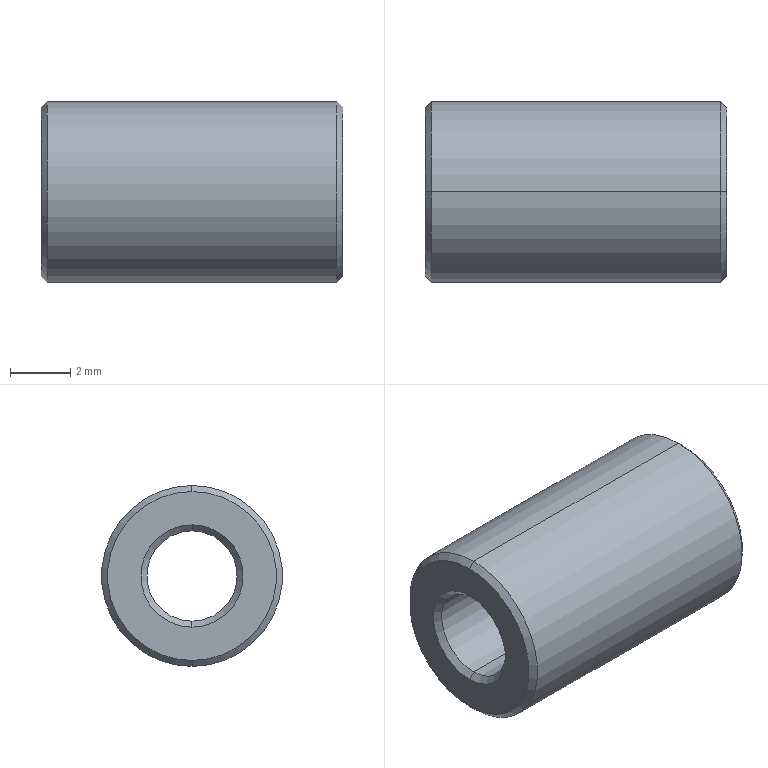Part | STEP file | KNCLSS3-8-10 | 1 solid | 14 faces | box 10 x 6 x 6 mm | volume 210.927 mm3 | cone 8 | cylinder 4 | plane 2 | commonest cylinder face diameters 3 x2 6 x2
STEP:
#1=CARTESIAN_POINT('',(0.,0.,0.));
#2=DIRECTION('',(0.,0.,1.));
#3=DIRECTION('',(1.,0.,0.));
#4=AXIS2_PLACEMENT_3D('',#1,#2,#3);
#5=CARTESIAN_POINT('',(9.8,0.,-1.5));
#6=VERTEX_POINT('',#5);
#7=CARTESIAN_POINT('',(10.,0.,-1.7));
#8=VERTEX_POINT('',#7);
#9=CARTESIAN_POINT('',(9.8,0.,-1.5));
#10=DIRECTION('',(0.7071,0.,-0.7071));
#11=VECTOR('',#10,1.);
#12=LINE('',#9,#11);
#13=CARTESIAN_POINT('',(9.8,0.,0.));
#14=DIRECTION('',(1.,0.,0.));
#15=DIRECTION('',(0.,0.,-1.));
#16=AXIS2_PLACEMENT_3D('',#13,#14,#15);
#17=CONICAL_SURFACE('',#16,1.5,0.7854);
#18=CARTESIAN_POINT('',(6.283,0.));
#19=DIRECTION('',(0.,1.));
#20=VECTOR('',#19,1.);
#21=LINE('',#18,#20);
#22=(GEOMETRIC_REPRESENTATION_CONTEXT(2)PARAMETRIC_REPRESENTATION_CONTEXT()REPRESENTATION_CONTEXT('',''));
#23=DEFINITIONAL_REPRESENTATION('',(#21),#22);
#24=PCURVE('',#17,#23);
#25=CARTESIAN_POINT('',(9.8,0.,0.));
#26=DIRECTION('',(1.,0.,0.));
#27=DIRECTION('',(0.,0.,-1.));
#28=AXIS2_PLACEMENT_3D('',#25,#26,#27);
#29=CONICAL_SURFACE('',#28,1.5,0.7854);
#30=CARTESIAN_POINT('',(0.,0.));
#31=DIRECTION('',(0.,1.));
#32=VECTOR('',#31,1.);
#33=LINE('',#30,#32);
#34=(GEOMETRIC_REPRESENTATION_CONTEXT(2)PARAMETRIC_REPRESENTATION_CONTEXT()REPRESENTATION_CONTEXT('',''));
#35=DEFINITIONAL_REPRESENTATION('',(#33),#34);
#36=PCURVE('',#29,#35);
#37=SURFACE_CURVE('',#12,(#24,#36),.PCURVE_S1.);
#38=EDGE_CURVE('',#6,#8,#37,.T.);
#39=ORIENTED_EDGE('',*,*,#38,.T.);
#40=CARTESIAN_POINT('',(10.,0.,1.7));
#41=VERTEX_POINT('',#40);
#42=CARTESIAN_POINT('',(10.,0.,0.));
#43=DIRECTION('',(1.,0.,0.));
#44=DIRECTION('',(0.,0.,-1.));
#45=AXIS2_PLACEMENT_3D('',#42,#43,#44);
#46=CIRCLE('',#45,1.7);
#47=CARTESIAN_POINT('',(0.,0.2));
#48=DIRECTION('',(1.,0.));
#49=VECTOR('',#48,1.);
#50=LINE('',#47,#49);
#51=(GEOMETRIC_REPRESENTATION_CONTEXT(2)PARAMETRIC_REPRESENTATION_CONTEXT()REPRESENTATION_CONTEXT('',''));
#52=DEFINITIONAL_REPRESENTATION('',(#50),#51);
#53=PCURVE('',#17,#52);
#54=CARTESIAN_POINT('',(10.,3.8,0.));
#55=DIRECTION('',(-1.,0.,0.));
#56=DIRECTION('',(0.,0.,1.));
#57=AXIS2_PLACEMENT_3D('',#54,#55,#56);
#58=PLANE('',#57);
#59=CARTESIAN_POINT('',(-1.7,-3.8));
#60=CARTESIAN_POINT('',(-1.7,-0.8555));
#61=CARTESIAN_POINT('',(0.85,-2.328));
#62=CARTESIAN_POINT('',(3.4,-3.8));
#63=CARTESIAN_POINT('',(0.85,-5.272));
#64=CARTESIAN_POINT('',(-1.7,-6.744));
#65=CARTESIAN_POINT('',(-1.7,-3.8));
#66=(BOUNDED_CURVE()B_SPLINE_CURVE(2,(#59,#60,#61,#62,#63,#64,#65),.UNSPECIFIED.,.T.,.F.)B_SPLINE_CURVE_WITH_KNOTS((1,2,2,2,2,1),(-2.094,0.,2.094,4.189,6.283,8.378),.UNSPECIFIED.)CURVE()GEOMETRIC_REPRESENTATION_ITEM()RATIONAL_B_SPLINE_CURVE((1.,0.5,1.,0.5,1.,0.5,1.))REPRESENTATION_ITEM(''));
#67=(GEOMETRIC_REPRESENTATION_CONTEXT(2)PARAMETRIC_REPRESENTATION_CONTEXT()REPRESENTATION_CONTEXT('',''));
#68=DEFINITIONAL_REPRESENTATION('',(#66),#67);
#69=PCURVE('',#58,#68);
#70=SURFACE_CURVE('',#46,(#53,#69),.PCURVE_S1.);
#71=EDGE_CURVE('',#41,#8,#70,.T.);
#72=ORIENTED_EDGE('',*,*,#71,.F.);
#73=CARTESIAN_POINT('',(9.8,0.,1.5));
#74=VERTEX_POINT('',#73);
#75=CARTESIAN_POINT('',(9.8,0.,1.5));
#76=DIRECTION('',(0.7071,0.,0.7071));
#77=VECTOR('',#76,1.);
#78=LINE('',#75,#77);
#79=CARTESIAN_POINT('',(3.142,0.));
#80=DIRECTION('',(0.,1.));
#81=VECTOR('',#80,1.);
#82=LINE('',#79,#81);
#83=(GEOMETRIC_REPRESENTATION_CONTEXT(2)PARAMETRIC_REPRESENTATION_CONTEXT()REPRESENTATION_CONTEXT('',''));
#84=DEFINITIONAL_REPRESENTATION('',(#82),#83);
#85=PCURVE('',#17,#84);
#86=CARTESIAN_POINT('',(3.142,0.));
#87=DIRECTION('',(0.,1.));
#88=VECTOR('',#87,1.);
#89=LINE('',#86,#88);
#90=(GEOMETRIC_REPRESENTATION_CONTEXT(2)PARAMETRIC_REPRESENTATION_CONTEXT()REPRESENTATION_CONTEXT('',''));
#91=DEFINITIONAL_REPRESENTATION('',(#89),#90);
#92=PCURVE('',#29,#91);
#93=SURFACE_CURVE('',#78,(#85,#92),.PCURVE_S1.);
#94=EDGE_CURVE('',#74,#41,#93,.T.);
#95=ORIENTED_EDGE('',*,*,#94,.F.);
#96=CARTESIAN_POINT('',(9.8,0.,0.));
#97=DIRECTION('',(1.,0.,0.));
#98=DIRECTION('',(0.,0.,-1.));
#99=AXIS2_PLACEMENT_3D('',#96,#97,#98);
#100=CIRCLE('',#99,1.5);
#101=CARTESIAN_POINT('',(0.,0.));
#102=DIRECTION('',(1.,0.));
#103=VECTOR('',#102,1.);
#104=LINE('',#101,#103);
#105=(GEOMETRIC_REPRESENTATION_CONTEXT(2)PARAMETRIC_REPRESENTATION_CONTEXT()REPRESENTATION_CONTEXT('',''));
#106=DEFINITIONAL_REPRESENTATION('',(#104),#105);
#107=PCURVE('',#17,#106);
#108=CARTESIAN_POINT('',(10.,0.,0.));
#109=DIRECTION('',(1.,0.,0.));
#110=DIRECTION('',(0.,0.,-1.));
#111=AXIS2_PLACEMENT_3D('',#108,#109,#110);
#112=CYLINDRICAL_SURFACE('',#111,1.5);
#113=CARTESIAN_POINT('',(0.,-0.2));
#114=DIRECTION('',(1.,0.));
#115=VECTOR('',#114,1.);
#116=LINE('',#113,#115);
#117=(GEOMETRIC_REPRESENTATION_CONTEXT(2)PARAMETRIC_REPRESENTATION_CONTEXT()REPRESENTATION_CONTEXT('',''));
#118=DEFINITIONAL_REPRESENTATION('',(#116),#117);
#119=PCURVE('',#112,#118);
#120=SURFACE_CURVE('',#100,(#107,#119),.PCURVE_S1.);
#121=EDGE_CURVE('',#74,#6,#120,.T.);
#122=ORIENTED_EDGE('',*,*,#121,.T.);
#123=EDGE_LOOP('',(#39,#72,#95,#122));
#124=FACE_BOUND('',#123,.F.);
#125=ADVANCED_FACE('',(#124),#17,.F.);
#126=CARTESIAN_POINT('',(0.2,0.,-1.5));
#127=VERTEX_POINT('',#126);
#128=CARTESIAN_POINT('',(10.,0.,-1.5));
#129=DIRECTION('',(1.,0.,0.));
#130=VECTOR('',#129,1.);
#131=LINE('',#128,#130);
#132=CARTESIAN_POINT('',(6.283,0.));
#133=DIRECTION('',(0.,1.));
#134=VECTOR('',#133,1.);
#135=LINE('',#132,#134);
#136=(GEOMETRIC_REPRESENTATION_CONTEXT(2)PARAMETRIC_REPRESENTATION_CONTEXT()REPRESENTATION_CONTEXT('',''));
#137=DEFINITIONAL_REPRESENTATION('',(#135),#136);
#138=PCURVE('',#112,#137);
#139=CARTESIAN_POINT('',(10.,0.,0.));
#140=DIRECTION('',(1.,0.,0.));
#141=DIRECTION('',(0.,0.,-1.));
#142=AXIS2_PLACEMENT_3D('',#139,#140,#141);
#143=CYLINDRICAL_SURFACE('',#142,1.5);
#144=CARTESIAN_POINT('',(0.,0.));
#145=DIRECTION('',(0.,1.));
#146=VECTOR('',#145,1.);
#147=LINE('',#144,#146);
#148=(GEOMETRIC_REPRESENTATION_CONTEXT(2)PARAMETRIC_REPRESENTATION_CONTEXT()REPRESENTATION_CONTEXT('',''));
#149=DEFINITIONAL_REPRESENTATION('',(#147),#148);
#150=PCURVE('',#143,#149);
#151=SURFACE_CURVE('',#131,(#138,#150),.PCURVE_S1.);
#152=EDGE_CURVE('',#127,#6,#151,.T.);
#153=ORIENTED_EDGE('',*,*,#152,.T.);
#154=ORIENTED_EDGE('',*,*,#121,.F.);
#155=CARTESIAN_POINT('',(0.2,0.,1.5));
#156=VERTEX_POINT('',#155);
#157=CARTESIAN_POINT('',(10.,0.,1.5));
#158=DIRECTION('',(1.,0.,0.));
#159=VECTOR('',#158,1.);
#160=LINE('',#157,#159);
#161=CARTESIAN_POINT('',(3.142,0.));
#162=DIRECTION('',(0.,1.));
#163=VECTOR('',#162,1.);
#164=LINE('',#161,#163);
#165=(GEOMETRIC_REPRESENTATION_CONTEXT(2)PARAMETRIC_REPRESENTATION_CONTEXT()REPRESENTATION_CONTEXT('',''));
#166=DEFINITIONAL_REPRESENTATION('',(#164),#165);
#167=PCURVE('',#112,#166);
#168=CARTESIAN_POINT('',(3.142,0.));
#169=DIRECTION('',(0.,1.));
#170=VECTOR('',#169,1.);
#171=LINE('',#168,#170);
#172=(GEOMETRIC_REPRESENTATION_CONTEXT(2)PARAMETRIC_REPRESENTATION_CONTEXT()REPRESENTATION_CONTEXT('',''));
#173=DEFINITIONAL_REPRESENTATION('',(#171),#172);
#174=PCURVE('',#143,#173);
#175=SURFACE_CURVE('',#160,(#167,#174),.PCURVE_S1.);
#176=EDGE_CURVE('',#156,#74,#175,.T.);
#177=ORIENTED_EDGE('',*,*,#176,.F.);
#178=CARTESIAN_POINT('',(0.2,0.,0.));
#179=DIRECTION('',(1.,0.,0.));
#180=DIRECTION('',(0.,0.,-1.));
#181=AXIS2_PLACEMENT_3D('',#178,#179,#180);
#182=CIRCLE('',#181,1.5);
#183=CARTESIAN_POINT('',(0.,-9.8));
#184=DIRECTION('',(1.,0.));
#185=VECTOR('',#184,1.);
#186=LINE('',#183,#185);
#187=(GEOMETRIC_REPRESENTATION_CONTEXT(2)PARAMETRIC_REPRESENTATION_CONTEXT()REPRESENTATION_CONTEXT('',''));
#188=DEFINITIONAL_REPRESENTATION('',(#186),#187);
#189=PCURVE('',#112,#188);
#190=CARTESIAN_POINT('',(0.,0.,0.));
#191=DIRECTION('',(-1.,0.,0.));
#192=DIRECTION('',(0.,0.,1.));
#193=AXIS2_PLACEMENT_3D('',#190,#191,#192);
#194=CONICAL_SURFACE('',#193,1.7,0.7854);
#195=CARTESIAN_POINT('',(9.425,-0.2));
#196=DIRECTION('',(-1.,0.));
#197=VECTOR('',#196,1.);
#198=LINE('',#195,#197);
#199=(GEOMETRIC_REPRESENTATION_CONTEXT(2)PARAMETRIC_REPRESENTATION_CONTEXT()REPRESENTATION_CONTEXT('',''));
#200=DEFINITIONAL_REPRESENTATION('',(#198),#199);
#201=PCURVE('',#194,#200);
#202=SURFACE_CURVE('',#182,(#189,#201),.PCURVE_S1.);
#203=EDGE_CURVE('',#156,#127,#202,.T.);
#204=ORIENTED_EDGE('',*,*,#203,.T.);
#205=EDGE_LOOP('',(#153,#154,#177,#204));
#206=FACE_BOUND('',#205,.F.);
#207=ADVANCED_FACE('',(#206),#112,.F.);
#208=CARTESIAN_POINT('',(0.,0.,1.7));
#209=VERTEX_POINT('',#208);
#210=CARTESIAN_POINT('',(0.,0.,1.7));
#211=DIRECTION('',(-0.7071,0.,0.7071));
#212=VECTOR('',#211,1.);
#213=LINE('',#210,#212);
#214=CARTESIAN_POINT('',(6.283,0.));
#215=DIRECTION('',(0.,1.));
#216=VECTOR('',#215,1.);
#217=LINE('',#214,#216);
#218=(GEOMETRIC_REPRESENTATION_CONTEXT(2)PARAMETRIC_REPRESENTATION_CONTEXT()REPRESENTATION_CONTEXT('',''));
#219=DEFINITIONAL_REPRESENTATION('',(#217),#218);
#220=PCURVE('',#194,#219);
#221=CARTESIAN_POINT('',(0.,0.,0.));
#222=DIRECTION('',(-1.,0.,0.));
#223=DIRECTION('',(0.,0.,1.));
#224=AXIS2_PLACEMENT_3D('',#221,#222,#223);
#225=CONICAL_SURFACE('',#224,1.7,0.7854);
#226=CARTESIAN_POINT('',(0.,0.));
#227=DIRECTION('',(0.,1.));
#228=VECTOR('',#227,1.);
#229=LINE('',#226,#228);
#230=(GEOMETRIC_REPRESENTATION_CONTEXT(2)PARAMETRIC_REPRESENTATION_CONTEXT()REPRESENTATION_CONTEXT('',''));
#231=DEFINITIONAL_REPRESENTATION('',(#229),#230);
#232=PCURVE('',#225,#231);
#233=SURFACE_CURVE('',#213,(#220,#232),.PCURVE_S1.);
#234=EDGE_CURVE('',#156,#209,#233,.T.);
#235=ORIENTED_EDGE('',*,*,#234,.T.);
#236=CARTESIAN_POINT('',(0.,0.,-1.7));
#237=VERTEX_POINT('',#236);
#238=CARTESIAN_POINT('',(0.,0.,0.));
#239=DIRECTION('',(1.,0.,0.));
#240=DIRECTION('',(0.,0.,-1.));
#241=AXIS2_PLACEMENT_3D('',#238,#239,#240);
#242=CIRCLE('',#241,1.7);
#243=CARTESIAN_POINT('',(9.425,0.));
#244=DIRECTION('',(-1.,0.));
#245=VECTOR('',#244,1.);
#246=LINE('',#243,#245);
#247=(GEOMETRIC_REPRESENTATION_CONTEXT(2)PARAMETRIC_REPRESENTATION_CONTEXT()REPRESENTATION_CONTEXT('',''));
#248=DEFINITIONAL_REPRESENTATION('',(#246),#247);
#249=PCURVE('',#194,#248);
#250=CARTESIAN_POINT('',(0.,0.,0.));
#251=DIRECTION('',(1.,0.,0.));
#252=DIRECTION('',(0.,0.,-1.));
#253=AXIS2_PLACEMENT_3D('',#250,#251,#252);
#254=PLANE('',#253);
#255=CARTESIAN_POINT('',(0.,0.));
#256=DIRECTION('',(1.,0.));
#257=AXIS2_PLACEMENT_2D('',#255,#256);
#258=CIRCLE('',#257,1.7);
#259=(GEOMETRIC_REPRESENTATION_CONTEXT(2)PARAMETRIC_REPRESENTATION_CONTEXT()REPRESENTATION_CONTEXT('',''));
#260=DEFINITIONAL_REPRESENTATION('',(#258),#259);
#261=PCURVE('',#254,#260);
#262=SURFACE_CURVE('',#242,(#249,#261),.PCURVE_S1.);
#263=EDGE_CURVE('',#209,#237,#262,.T.);
#264=ORIENTED_EDGE('',*,*,#263,.T.);
#265=CARTESIAN_POINT('',(0.,0.,-1.7));
#266=DIRECTION('',(-0.7071,0.,-0.7071));
#267=VECTOR('',#266,1.);
#268=LINE('',#265,#267);
#269=CARTESIAN_POINT('',(3.142,0.));
#270=DIRECTION('',(0.,1.));
#271=VECTOR('',#270,1.);
#272=LINE('',#269,#271);
#273=(GEOMETRIC_REPRESENTATION_CONTEXT(2)PARAMETRIC_REPRESENTATION_CONTEXT()REPRESENTATION_CONTEXT('',''));
#274=DEFINITIONAL_REPRESENTATION('',(#272),#273);
#275=PCURVE('',#194,#274);
#276=CARTESIAN_POINT('',(3.142,0.));
#277=DIRECTION('',(0.,1.));
#278=VECTOR('',#277,1.);
#279=LINE('',#276,#278);
#280=(GEOMETRIC_REPRESENTATION_CONTEXT(2)PARAMETRIC_REPRESENTATION_CONTEXT()REPRESENTATION_CONTEXT('',''));
#281=DEFINITIONAL_REPRESENTATION('',(#279),#280);
#282=PCURVE('',#225,#281);
#283=SURFACE_CURVE('',#268,(#275,#282),.PCURVE_S1.);
#284=EDGE_CURVE('',#127,#237,#283,.T.);
#285=ORIENTED_EDGE('',*,*,#284,.F.);
#286=ORIENTED_EDGE('',*,*,#203,.F.);
#287=EDGE_LOOP('',(#235,#264,#285,#286));
#288=FACE_BOUND('',#287,.F.);
#289=ADVANCED_FACE('',(#288),#194,.F.);
#290=CARTESIAN_POINT('',(10.,0.,-2.8));
#291=VERTEX_POINT('',#290);
#292=CARTESIAN_POINT('',(10.,0.,2.8));
#293=VERTEX_POINT('',#292);
#294=CARTESIAN_POINT('',(10.,0.,0.));
#295=DIRECTION('',(1.,0.,0.));
#296=DIRECTION('',(0.,0.,1.));
#297=AXIS2_PLACEMENT_3D('',#294,#295,#296);
#298=CIRCLE('',#297,2.8);
#299=CARTESIAN_POINT('',(9.8,0.,0.));
#300=DIRECTION('',(-1.,0.,0.));
#301=DIRECTION('',(0.,0.,1.));
#302=AXIS2_PLACEMENT_3D('',#299,#300,#301);
#303=CONICAL_SURFACE('',#302,3.,0.7854);
#304=CARTESIAN_POINT('',(6.283,-0.2));
#305=DIRECTION('',(-1.,0.));
#306=VECTOR('',#305,1.);
#307=LINE('',#304,#306);
#308=(GEOMETRIC_REPRESENTATION_CONTEXT(2)PARAMETRIC_REPRESENTATION_CONTEXT()REPRESENTATION_CONTEXT('',''));
#309=DEFINITIONAL_REPRESENTATION('',(#307),#308);
#310=PCURVE('',#303,#309);
#311=CARTESIAN_POINT('',(2.8,-3.8));
#312=CARTESIAN_POINT('',(2.8,-8.65));
#313=CARTESIAN_POINT('',(-1.4,-6.225));
#314=CARTESIAN_POINT('',(-5.6,-3.8));
#315=CARTESIAN_POINT('',(-1.4,-1.375));
#316=CARTESIAN_POINT('',(2.8,1.05));
#317=CARTESIAN_POINT('',(2.8,-3.8));
#318=(BOUNDED_CURVE()B_SPLINE_CURVE(2,(#311,#312,#313,#314,#315,#316,#317),.UNSPECIFIED.,.T.,.F.)B_SPLINE_CURVE_WITH_KNOTS((1,2,2,2,2,1),(-2.094,0.,2.094,4.189,6.283,8.378),.UNSPECIFIED.)CURVE()GEOMETRIC_REPRESENTATION_ITEM()RATIONAL_B_SPLINE_CURVE((1.,0.5,1.,0.5,1.,0.5,1.))REPRESENTATION_ITEM(''));
#319=(GEOMETRIC_REPRESENTATION_CONTEXT(2)PARAMETRIC_REPRESENTATION_CONTEXT()REPRESENTATION_CONTEXT('',''));
#320=DEFINITIONAL_REPRESENTATION('',(#318),#319);
#321=PCURVE('',#58,#320);
#322=SURFACE_CURVE('',#298,(#310,#321),.PCURVE_S1.);
#323=EDGE_CURVE('',#291,#293,#322,.T.);
#324=ORIENTED_EDGE('',*,*,#323,.F.);
#325=CARTESIAN_POINT('',(9.8,0.,-3.));
#326=VERTEX_POINT('',#325);
#327=CARTESIAN_POINT('',(9.8,0.,-3.));
#328=DIRECTION('',(-0.7071,0.,-0.7071));
#329=VECTOR('',#328,1.);
#330=LINE('',#327,#329);
#331=CARTESIAN_POINT('',(3.142,0.));
#332=DIRECTION('',(0.,1.));
#333=VECTOR('',#332,1.);
#334=LINE('',#331,#333);
#335=(GEOMETRIC_REPRESENTATION_CONTEXT(2)PARAMETRIC_REPRESENTATION_CONTEXT()REPRESENTATION_CONTEXT('',''));
#336=DEFINITIONAL_REPRESENTATION('',(#334),#335);
#337=PCURVE('',#303,#336);
#338=CARTESIAN_POINT('',(9.8,0.,0.));
#339=DIRECTION('',(-1.,0.,0.));
#340=DIRECTION('',(0.,0.,1.));
#341=AXIS2_PLACEMENT_3D('',#338,#339,#340);
#342=CONICAL_SURFACE('',#341,3.,0.7854);
#343=CARTESIAN_POINT('',(3.142,0.));
#344=DIRECTION('',(0.,1.));
#345=VECTOR('',#344,1.);
#346=LINE('',#343,#345);
#347=(GEOMETRIC_REPRESENTATION_CONTEXT(2)PARAMETRIC_REPRESENTATION_CONTEXT()REPRESENTATION_CONTEXT('',''));
#348=DEFINITIONAL_REPRESENTATION('',(#346),#347);
#349=PCURVE('',#342,#348);
#350=SURFACE_CURVE('',#330,(#337,#349),.PCURVE_S1.);
#351=EDGE_CURVE('',#291,#326,#350,.T.);
#352=ORIENTED_EDGE('',*,*,#351,.T.);
#353=CARTESIAN_POINT('',(9.8,0.,3.));
#354=VERTEX_POINT('',#353);
#355=CARTESIAN_POINT('',(9.8,0.,0.));
#356=DIRECTION('',(1.,0.,0.));
#357=DIRECTION('',(0.,0.,1.));
#358=AXIS2_PLACEMENT_3D('',#355,#356,#357);
#359=CIRCLE('',#358,3.);
#360=CARTESIAN_POINT('',(6.283,0.));
#361=DIRECTION('',(-1.,0.));
#362=VECTOR('',#361,1.);
#363=LINE('',#360,#362);
#364=(GEOMETRIC_REPRESENTATION_CONTEXT(2)PARAMETRIC_REPRESENTATION_CONTEXT()REPRESENTATION_CONTEXT('',''));
#365=DEFINITIONAL_REPRESENTATION('',(#363),#364);
#366=PCURVE('',#303,#365);
#367=CARTESIAN_POINT('',(10.,0.,0.));
#368=DIRECTION('',(1.,0.,0.));
#369=DIRECTION('',(0.,0.,-1.));
#370=AXIS2_PLACEMENT_3D('',#367,#368,#369);
#371=CYLINDRICAL_SURFACE('',#370,3.);
#372=CARTESIAN_POINT('',(-3.142,-0.2));
#373=DIRECTION('',(1.,0.));
#374=VECTOR('',#373,1.);
#375=LINE('',#372,#374);
#376=(GEOMETRIC_REPRESENTATION_CONTEXT(2)PARAMETRIC_REPRESENTATION_CONTEXT()REPRESENTATION_CONTEXT('',''));
#377=DEFINITIONAL_REPRESENTATION('',(#375),#376);
#378=PCURVE('',#371,#377);
#379=SURFACE_CURVE('',#359,(#366,#378),.PCURVE_S1.);
#380=EDGE_CURVE('',#326,#354,#379,.T.);
#381=ORIENTED_EDGE('',*,*,#380,.T.);
#382=CARTESIAN_POINT('',(9.8,0.,3.));
#383=DIRECTION('',(-0.7071,0.,0.7071));
#384=VECTOR('',#383,1.);
#385=LINE('',#382,#384);
#386=CARTESIAN_POINT('',(0.,0.));
#387=DIRECTION('',(0.,1.));
#388=VECTOR('',#387,1.);
#389=LINE('',#386,#388);
#390=(GEOMETRIC_REPRESENTATION_CONTEXT(2)PARAMETRIC_REPRESENTATION_CONTEXT()REPRESENTATION_CONTEXT('',''));
#391=DEFINITIONAL_REPRESENTATION('',(#389),#390);
#392=PCURVE('',#303,#391);
#393=CARTESIAN_POINT('',(6.283,0.));
#394=DIRECTION('',(0.,1.));
#395=VECTOR('',#394,1.);
#396=LINE('',#393,#395);
#397=(GEOMETRIC_REPRESENTATION_CONTEXT(2)PARAMETRIC_REPRESENTATION_CONTEXT()REPRESENTATION_CONTEXT('',''));
#398=DEFINITIONAL_REPRESENTATION('',(#396),#397);
#399=PCURVE('',#342,#398);
#400=SURFACE_CURVE('',#385,(#392,#399),.PCURVE_S1.);
#401=EDGE_CURVE('',#293,#354,#400,.T.);
#402=ORIENTED_EDGE('',*,*,#401,.F.);
#403=EDGE_LOOP('',(#324,#352,#381,#402));
#404=FACE_BOUND('',#403,.T.);
#405=ADVANCED_FACE('',(#404),#303,.T.);
#406=CARTESIAN_POINT('',(0.2,0.,-3.));
#407=VERTEX_POINT('',#406);
#408=CARTESIAN_POINT('',(0.2,0.,3.));
#409=VERTEX_POINT('',#408);
#410=CARTESIAN_POINT('',(0.2,0.,0.));
#411=DIRECTION('',(1.,0.,0.));
#412=DIRECTION('',(0.,0.,-1.));
#413=AXIS2_PLACEMENT_3D('',#410,#411,#412);
#414=CIRCLE('',#413,3.);
#415=CARTESIAN_POINT('',(0.,-9.8));
#416=DIRECTION('',(1.,0.));
#417=VECTOR('',#416,1.);
#418=LINE('',#415,#417);
#419=(GEOMETRIC_REPRESENTATION_CONTEXT(2)PARAMETRIC_REPRESENTATION_CONTEXT()REPRESENTATION_CONTEXT('',''));
#420=DEFINITIONAL_REPRESENTATION('',(#418),#419);
#421=PCURVE('',#371,#420);
#422=CARTESIAN_POINT('',(0.,0.,0.));
#423=DIRECTION('',(1.,0.,0.));
#424=DIRECTION('',(0.,0.,-1.));
#425=AXIS2_PLACEMENT_3D('',#422,#423,#424);
#426=CONICAL_SURFACE('',#425,2.8,0.7854);
#427=CARTESIAN_POINT('',(0.,0.2));
#428=DIRECTION('',(1.,0.));
#429=VECTOR('',#428,1.);
#430=LINE('',#427,#429);
#431=(GEOMETRIC_REPRESENTATION_CONTEXT(2)PARAMETRIC_REPRESENTATION_CONTEXT()REPRESENTATION_CONTEXT('',''));
#432=DEFINITIONAL_REPRESENTATION('',(#430),#431);
#433=PCURVE('',#426,#432);
#434=SURFACE_CURVE('',#414,(#421,#433),.PCURVE_S1.);
#435=EDGE_CURVE('',#407,#409,#434,.T.);
#436=ORIENTED_EDGE('',*,*,#435,.T.);
#437=CARTESIAN_POINT('',(10.,0.,3.));
#438=DIRECTION('',(1.,0.,0.));
#439=VECTOR('',#438,1.);
#440=LINE('',#437,#439);
#441=CARTESIAN_POINT('',(3.142,0.));
#442=DIRECTION('',(0.,1.));
#443=VECTOR('',#442,1.);
#444=LINE('',#441,#443);
#445=(GEOMETRIC_REPRESENTATION_CONTEXT(2)PARAMETRIC_REPRESENTATION_CONTEXT()REPRESENTATION_CONTEXT('',''));
#446=DEFINITIONAL_REPRESENTATION('',(#444),#445);
#447=PCURVE('',#371,#446);
#448=CARTESIAN_POINT('',(10.,0.,0.));
#449=DIRECTION('',(1.,0.,0.));
#450=DIRECTION('',(0.,0.,-1.));
#451=AXIS2_PLACEMENT_3D('',#448,#449,#450);
#452=CYLINDRICAL_SURFACE('',#451,3.);
#453=CARTESIAN_POINT('',(3.142,0.));
#454=DIRECTION('',(0.,1.));
#455=VECTOR('',#454,1.);
#456=LINE('',#453,#455);
#457=(GEOMETRIC_REPRESENTATION_CONTEXT(2)PARAMETRIC_REPRESENTATION_CONTEXT()REPRESENTATION_CONTEXT('',''));
#458=DEFINITIONAL_REPRESENTATION('',(#456),#457);
#459=PCURVE('',#452,#458);
#460=SURFACE_CURVE('',#440,(#447,#459),.PCURVE_S1.);
#461=EDGE_CURVE('',#409,#354,#460,.T.);
#462=ORIENTED_EDGE('',*,*,#461,.T.);
#463=ORIENTED_EDGE('',*,*,#380,.F.);
#464=CARTESIAN_POINT('',(10.,0.,-3.));
#465=DIRECTION('',(1.,0.,0.));
#466=VECTOR('',#465,1.);
#467=LINE('',#464,#466);
#468=CARTESIAN_POINT('',(0.,0.));
#469=DIRECTION('',(0.,1.));
#470=VECTOR('',#469,1.);
#471=LINE('',#468,#470);
#472=(GEOMETRIC_REPRESENTATION_CONTEXT(2)PARAMETRIC_REPRESENTATION_CONTEXT()REPRESENTATION_CONTEXT('',''));
#473=DEFINITIONAL_REPRESENTATION('',(#471),#472);
#474=PCURVE('',#371,#473);
#475=CARTESIAN_POINT('',(6.283,0.));
#476=DIRECTION('',(0.,1.));
#477=VECTOR('',#476,1.);
#478=LINE('',#475,#477);
#479=(GEOMETRIC_REPRESENTATION_CONTEXT(2)PARAMETRIC_REPRESENTATION_CONTEXT()REPRESENTATION_CONTEXT('',''));
#480=DEFINITIONAL_REPRESENTATION('',(#478),#479);
#481=PCURVE('',#452,#480);
#482=SURFACE_CURVE('',#467,(#474,#481),.PCURVE_S1.);
#483=EDGE_CURVE('',#407,#326,#482,.T.);
#484=ORIENTED_EDGE('',*,*,#483,.F.);
#485=EDGE_LOOP('',(#436,#462,#463,#484));
#486=FACE_BOUND('',#485,.T.);
#487=ADVANCED_FACE('',(#486),#371,.T.);
#488=CARTESIAN_POINT('',(0.,0.,-2.8));
#489=VERTEX_POINT('',#488);
#490=CARTESIAN_POINT('',(0.,0.,2.8));
#491=VERTEX_POINT('',#490);
#492=CARTESIAN_POINT('',(0.,0.,0.));
#493=DIRECTION('',(1.,0.,0.));
#494=DIRECTION('',(0.,0.,-1.));
#495=AXIS2_PLACEMENT_3D('',#492,#493,#494);
#496=CIRCLE('',#495,2.8);
#497=CARTESIAN_POINT('',(0.,0.));
#498=DIRECTION('',(1.,0.));
#499=VECTOR('',#498,1.);
#500=LINE('',#497,#499);
#501=(GEOMETRIC_REPRESENTATION_CONTEXT(2)PARAMETRIC_REPRESENTATION_CONTEXT()REPRESENTATION_CONTEXT('',''));
#502=DEFINITIONAL_REPRESENTATION('',(#500),#501);
#503=PCURVE('',#426,#502);
#504=CARTESIAN_POINT('',(0.,0.));
#505=DIRECTION('',(1.,0.));
#506=AXIS2_PLACEMENT_2D('',#504,#505);
#507=CIRCLE('',#506,2.8);
#508=(GEOMETRIC_REPRESENTATION_CONTEXT(2)PARAMETRIC_REPRESENTATION_CONTEXT()REPRESENTATION_CONTEXT('',''));
#509=DEFINITIONAL_REPRESENTATION('',(#507),#508);
#510=PCURVE('',#254,#509);
#511=SURFACE_CURVE('',#496,(#503,#510),.PCURVE_S1.);
#512=EDGE_CURVE('',#489,#491,#511,.T.);
#513=ORIENTED_EDGE('',*,*,#512,.T.);
#514=CARTESIAN_POINT('',(0.,0.,2.8));
#515=DIRECTION('',(0.7071,0.,0.7071));
#516=VECTOR('',#515,1.);
#517=LINE('',#514,#516);
#518=CARTESIAN_POINT('',(3.142,0.));
#519=DIRECTION('',(0.,1.));
#520=VECTOR('',#519,1.);
#521=LINE('',#518,#520);
#522=(GEOMETRIC_REPRESENTATION_CONTEXT(2)PARAMETRIC_REPRESENTATION_CONTEXT()REPRESENTATION_CONTEXT('',''));
#523=DEFINITIONAL_REPRESENTATION('',(#521),#522);
#524=PCURVE('',#426,#523);
#525=CARTESIAN_POINT('',(0.,0.,0.));
#526=DIRECTION('',(1.,0.,0.));
#527=DIRECTION('',(0.,0.,-1.));
#528=AXIS2_PLACEMENT_3D('',#525,#526,#527);
#529=CONICAL_SURFACE('',#528,2.8,0.7854);
#530=CARTESIAN_POINT('',(3.142,0.));
#531=DIRECTION('',(0.,1.));
#532=VECTOR('',#531,1.);
#533=LINE('',#530,#532);
#534=(GEOMETRIC_REPRESENTATION_CONTEXT(2)PARAMETRIC_REPRESENTATION_CONTEXT()REPRESENTATION_CONTEXT('',''));
#535=DEFINITIONAL_REPRESENTATION('',(#533),#534);
#536=PCURVE('',#529,#535);
#537=SURFACE_CURVE('',#517,(#524,#536),.PCURVE_S1.);
#538=EDGE_CURVE('',#491,#409,#537,.T.);
#539=ORIENTED_EDGE('',*,*,#538,.T.);
#540=ORIENTED_EDGE('',*,*,#435,.F.);
#541=CARTESIAN_POINT('',(0.,0.,-2.8));
#542=DIRECTION('',(0.7071,0.,-0.7071));
#543=VECTOR('',#542,1.);
#544=LINE('',#541,#543);
#545=CARTESIAN_POINT('',(0.,0.));
#546=DIRECTION('',(0.,1.));
#547=VECTOR('',#546,1.);
#548=LINE('',#545,#547);
#549=(GEOMETRIC_REPRESENTATION_CONTEXT(2)PARAMETRIC_REPRESENTATION_CONTEXT()REPRESENTATION_CONTEXT('',''));
#550=DEFINITIONAL_REPRESENTATION('',(#548),#549);
#551=PCURVE('',#426,#550);
#552=CARTESIAN_POINT('',(6.283,0.));
#553=DIRECTION('',(0.,1.));
#554=VECTOR('',#553,1.);
#555=LINE('',#552,#554);
#556=(GEOMETRIC_REPRESENTATION_CONTEXT(2)PARAMETRIC_REPRESENTATION_CONTEXT()REPRESENTATION_CONTEXT('',''));
#557=DEFINITIONAL_REPRESENTATION('',(#555),#556);
#558=PCURVE('',#529,#557);
#559=SURFACE_CURVE('',#544,(#551,#558),.PCURVE_S1.);
#560=EDGE_CURVE('',#489,#407,#559,.T.);
#561=ORIENTED_EDGE('',*,*,#560,.F.);
#562=EDGE_LOOP('',(#513,#539,#540,#561));
#563=FACE_BOUND('',#562,.T.);
#564=ADVANCED_FACE('',(#563),#426,.T.);
#565=ORIENTED_EDGE('',*,*,#512,.F.);
#566=CARTESIAN_POINT('',(0.,0.,0.));
#567=DIRECTION('',(1.,0.,0.));
#568=DIRECTION('',(0.,0.,-1.));
#569=AXIS2_PLACEMENT_3D('',#566,#567,#568);
#570=CIRCLE('',#569,2.8);
#571=CARTESIAN_POINT('',(0.,0.));
#572=DIRECTION('',(1.,0.));
#573=AXIS2_PLACEMENT_2D('',#571,#572);
#574=CIRCLE('',#573,2.8);
#575=(GEOMETRIC_REPRESENTATION_CONTEXT(2)PARAMETRIC_REPRESENTATION_CONTEXT()REPRESENTATION_CONTEXT('',''));
#576=DEFINITIONAL_REPRESENTATION('',(#574),#575);
#577=PCURVE('',#254,#576);
#578=CARTESIAN_POINT('',(0.,0.));
#579=DIRECTION('',(1.,0.));
#580=VECTOR('',#579,1.);
#581=LINE('',#578,#580);
#582=(GEOMETRIC_REPRESENTATION_CONTEXT(2)PARAMETRIC_REPRESENTATION_CONTEXT()REPRESENTATION_CONTEXT('',''));
#583=DEFINITIONAL_REPRESENTATION('',(#581),#582);
#584=PCURVE('',#529,#583);
#585=SURFACE_CURVE('',#570,(#577,#584),.PCURVE_S1.);
#586=EDGE_CURVE('',#491,#489,#585,.T.);
#587=ORIENTED_EDGE('',*,*,#586,.F.);
#588=EDGE_LOOP('',(#565,#587));
#589=FACE_BOUND('',#588,.T.);
#590=ORIENTED_EDGE('',*,*,#263,.T.);
#591=CARTESIAN_POINT('',(0.,0.,0.));
#592=DIRECTION('',(1.,0.,0.));
#593=DIRECTION('',(0.,0.,-1.));
#594=AXIS2_PLACEMENT_3D('',#591,#592,#593);
#595=CIRCLE('',#594,1.7);
#596=CARTESIAN_POINT('',(0.,0.));
#597=DIRECTION('',(1.,0.));
#598=AXIS2_PLACEMENT_2D('',#596,#597);
#599=CIRCLE('',#598,1.7);
#600=(GEOMETRIC_REPRESENTATION_CONTEXT(2)PARAMETRIC_REPRESENTATION_CONTEXT()REPRESENTATION_CONTEXT('',''));
#601=DEFINITIONAL_REPRESENTATION('',(#599),#600);
#602=PCURVE('',#254,#601);
#603=CARTESIAN_POINT('',(3.142,0.));
#604=DIRECTION('',(-1.,0.));
#605=VECTOR('',#604,1.);
#606=LINE('',#603,#605);
#607=(GEOMETRIC_REPRESENTATION_CONTEXT(2)PARAMETRIC_REPRESENTATION_CONTEXT()REPRESENTATION_CONTEXT('',''));
#608=DEFINITIONAL_REPRESENTATION('',(#606),#607);
#609=PCURVE('',#225,#608);
#610=SURFACE_CURVE('',#595,(#602,#609),.PCURVE_S1.);
#611=EDGE_CURVE('',#237,#209,#610,.T.);
#612=ORIENTED_EDGE('',*,*,#611,.T.);
#613=EDGE_LOOP('',(#590,#612));
#614=FACE_BOUND('',#613,.T.);
#615=ADVANCED_FACE('',(#589,#614),#254,.F.);
#616=ORIENTED_EDGE('',*,*,#538,.F.);
#617=ORIENTED_EDGE('',*,*,#586,.T.);
#618=ORIENTED_EDGE('',*,*,#560,.T.);
#619=CARTESIAN_POINT('',(0.2,0.,0.));
#620=DIRECTION('',(1.,0.,0.));
#621=DIRECTION('',(0.,0.,-1.));
#622=AXIS2_PLACEMENT_3D('',#619,#620,#621);
#623=CIRCLE('',#622,3.);
#624=CARTESIAN_POINT('',(0.,0.2));
#625=DIRECTION('',(1.,0.));
#626=VECTOR('',#625,1.);
#627=LINE('',#624,#626);
#628=(GEOMETRIC_REPRESENTATION_CONTEXT(2)PARAMETRIC_REPRESENTATION_CONTEXT()REPRESENTATION_CONTEXT('',''));
#629=DEFINITIONAL_REPRESENTATION('',(#627),#628);
#630=PCURVE('',#529,#629);
#631=CARTESIAN_POINT('',(0.,-9.8));
#632=DIRECTION('',(1.,0.));
#633=VECTOR('',#632,1.);
#634=LINE('',#631,#633);
#635=(GEOMETRIC_REPRESENTATION_CONTEXT(2)PARAMETRIC_REPRESENTATION_CONTEXT()REPRESENTATION_CONTEXT('',''));
#636=DEFINITIONAL_REPRESENTATION('',(#634),#635);
#637=PCURVE('',#452,#636);
#638=SURFACE_CURVE('',#623,(#630,#637),.PCURVE_S1.);
#639=EDGE_CURVE('',#409,#407,#638,.T.);
#640=ORIENTED_EDGE('',*,*,#639,.F.);
#641=EDGE_LOOP('',(#616,#617,#618,#640));
#642=FACE_BOUND('',#641,.T.);
#643=ADVANCED_FACE('',(#642),#529,.T.);
#644=ORIENTED_EDGE('',*,*,#461,.F.);
#645=ORIENTED_EDGE('',*,*,#639,.T.);
#646=ORIENTED_EDGE('',*,*,#483,.T.);
#647=CARTESIAN_POINT('',(9.8,0.,0.));
#648=DIRECTION('',(1.,0.,0.));
#649=DIRECTION('',(0.,0.,1.));
#650=AXIS2_PLACEMENT_3D('',#647,#648,#649);
#651=CIRCLE('',#650,3.);
#652=CARTESIAN_POINT('',(3.142,-0.2));
#653=DIRECTION('',(1.,0.));
#654=VECTOR('',#653,1.);
#655=LINE('',#652,#654);
#656=(GEOMETRIC_REPRESENTATION_CONTEXT(2)PARAMETRIC_REPRESENTATION_CONTEXT()REPRESENTATION_CONTEXT('',''));
#657=DEFINITIONAL_REPRESENTATION('',(#655),#656);
#658=PCURVE('',#452,#657);
#659=CARTESIAN_POINT('',(6.283,0.));
#660=DIRECTION('',(-1.,0.));
#661=VECTOR('',#660,1.);
#662=LINE('',#659,#661);
#663=(GEOMETRIC_REPRESENTATION_CONTEXT(2)PARAMETRIC_REPRESENTATION_CONTEXT()REPRESENTATION_CONTEXT('',''));
#664=DEFINITIONAL_REPRESENTATION('',(#662),#663);
#665=PCURVE('',#342,#664);
#666=SURFACE_CURVE('',#651,(#658,#665),.PCURVE_S1.);
#667=EDGE_CURVE('',#354,#326,#666,.T.);
#668=ORIENTED_EDGE('',*,*,#667,.F.);
#669=EDGE_LOOP('',(#644,#645,#646,#668));
#670=FACE_BOUND('',#669,.T.);
#671=ADVANCED_FACE('',(#670),#452,.T.);
#672=ORIENTED_EDGE('',*,*,#351,.F.);
#673=CARTESIAN_POINT('',(10.,0.,0.));
#674=DIRECTION('',(1.,0.,0.));
#675=DIRECTION('',(0.,0.,1.));
#676=AXIS2_PLACEMENT_3D('',#673,#674,#675);
#677=CIRCLE('',#676,2.8);
#678=CARTESIAN_POINT('',(6.283,-0.2));
#679=DIRECTION('',(-1.,0.));
#680=VECTOR('',#679,1.);
#681=LINE('',#678,#680);
#682=(GEOMETRIC_REPRESENTATION_CONTEXT(2)PARAMETRIC_REPRESENTATION_CONTEXT()REPRESENTATION_CONTEXT('',''));
#683=DEFINITIONAL_REPRESENTATION('',(#681),#682);
#684=PCURVE('',#342,#683);
#685=CARTESIAN_POINT('',(2.8,-3.8));
#686=CARTESIAN_POINT('',(2.8,-8.65));
#687=CARTESIAN_POINT('',(-1.4,-6.225));
#688=CARTESIAN_POINT('',(-5.6,-3.8));
#689=CARTESIAN_POINT('',(-1.4,-1.375));
#690=CARTESIAN_POINT('',(2.8,1.05));
#691=CARTESIAN_POINT('',(2.8,-3.8));
#692=(BOUNDED_CURVE()B_SPLINE_CURVE(2,(#685,#686,#687,#688,#689,#690,#691),.UNSPECIFIED.,.T.,.F.)B_SPLINE_CURVE_WITH_KNOTS((1,2,2,2,2,1),(-2.094,0.,2.094,4.189,6.283,8.378),.UNSPECIFIED.)CURVE()GEOMETRIC_REPRESENTATION_ITEM()RATIONAL_B_SPLINE_CURVE((1.,0.5,1.,0.5,1.,0.5,1.))REPRESENTATION_ITEM(''));
#693=(GEOMETRIC_REPRESENTATION_CONTEXT(2)PARAMETRIC_REPRESENTATION_CONTEXT()REPRESENTATION_CONTEXT('',''));
#694=DEFINITIONAL_REPRESENTATION('',(#692),#693);
#695=PCURVE('',#58,#694);
#696=SURFACE_CURVE('',#677,(#684,#695),.PCURVE_S1.);
#697=EDGE_CURVE('',#293,#291,#696,.T.);
#698=ORIENTED_EDGE('',*,*,#697,.F.);
#699=ORIENTED_EDGE('',*,*,#401,.T.);
#700=ORIENTED_EDGE('',*,*,#667,.T.);
#701=EDGE_LOOP('',(#672,#698,#699,#700));
#702=FACE_BOUND('',#701,.T.);
#703=ADVANCED_FACE('',(#702),#342,.T.);
#704=CARTESIAN_POINT('',(10.,0.,0.));
#705=DIRECTION('',(1.,0.,0.));
#706=DIRECTION('',(0.,0.,-1.));
#707=AXIS2_PLACEMENT_3D('',#704,#705,#706);
#708=CIRCLE('',#707,1.7);
#709=CARTESIAN_POINT('',(-1.7,-3.8));
#710=CARTESIAN_POINT('',(-1.7,-0.8555));
#711=CARTESIAN_POINT('',(0.85,-2.328));
#712=CARTESIAN_POINT('',(3.4,-3.8));
#713=CARTESIAN_POINT('',(0.85,-5.272));
#714=CARTESIAN_POINT('',(-1.7,-6.744));
#715=CARTESIAN_POINT('',(-1.7,-3.8));
#716=(BOUNDED_CURVE()B_SPLINE_CURVE(2,(#709,#710,#711,#712,#713,#714,#715),.UNSPECIFIED.,.T.,.F.)B_SPLINE_CURVE_WITH_KNOTS((1,2,2,2,2,1),(-2.094,0.,2.094,4.189,6.283,8.378),.UNSPECIFIED.)CURVE()GEOMETRIC_REPRESENTATION_ITEM()RATIONAL_B_SPLINE_CURVE((1.,0.5,1.,0.5,1.,0.5,1.))REPRESENTATION_ITEM(''));
#717=(GEOMETRIC_REPRESENTATION_CONTEXT(2)PARAMETRIC_REPRESENTATION_CONTEXT()REPRESENTATION_CONTEXT('',''));
#718=DEFINITIONAL_REPRESENTATION('',(#716),#717);
#719=PCURVE('',#58,#718);
#720=CARTESIAN_POINT('',(0.,0.2));
#721=DIRECTION('',(1.,0.));
#722=VECTOR('',#721,1.);
#723=LINE('',#720,#722);
#724=(GEOMETRIC_REPRESENTATION_CONTEXT(2)PARAMETRIC_REPRESENTATION_CONTEXT()REPRESENTATION_CONTEXT('',''));
#725=DEFINITIONAL_REPRESENTATION('',(#723),#724);
#726=PCURVE('',#29,#725);
#727=SURFACE_CURVE('',#708,(#719,#726),.PCURVE_S1.);
#728=EDGE_CURVE('',#8,#41,#727,.T.);
#729=ORIENTED_EDGE('',*,*,#728,.F.);
#730=ORIENTED_EDGE('',*,*,#71,.F.);
#731=EDGE_LOOP('',(#729,#730));
#732=FACE_BOUND('',#731,.T.);
#733=ORIENTED_EDGE('',*,*,#697,.T.);
#734=ORIENTED_EDGE('',*,*,#323,.T.);
#735=EDGE_LOOP('',(#733,#734));
#736=FACE_BOUND('',#735,.T.);
#737=ADVANCED_FACE('',(#732,#736),#58,.F.);
#738=ORIENTED_EDGE('',*,*,#611,.T.);
#739=ORIENTED_EDGE('',*,*,#234,.F.);
#740=CARTESIAN_POINT('',(0.2,0.,0.));
#741=DIRECTION('',(1.,0.,0.));
#742=DIRECTION('',(0.,0.,-1.));
#743=AXIS2_PLACEMENT_3D('',#740,#741,#742);
#744=CIRCLE('',#743,1.5);
#745=CARTESIAN_POINT('',(3.142,-0.2));
#746=DIRECTION('',(-1.,0.));
#747=VECTOR('',#746,1.);
#748=LINE('',#745,#747);
#749=(GEOMETRIC_REPRESENTATION_CONTEXT(2)PARAMETRIC_REPRESENTATION_CONTEXT()REPRESENTATION_CONTEXT('',''));
#750=DEFINITIONAL_REPRESENTATION('',(#748),#749);
#751=PCURVE('',#225,#750);
#752=CARTESIAN_POINT('',(0.,-9.8));
#753=DIRECTION('',(1.,0.));
#754=VECTOR('',#753,1.);
#755=LINE('',#752,#754);
#756=(GEOMETRIC_REPRESENTATION_CONTEXT(2)PARAMETRIC_REPRESENTATION_CONTEXT()REPRESENTATION_CONTEXT('',''));
#757=DEFINITIONAL_REPRESENTATION('',(#755),#756);
#758=PCURVE('',#143,#757);
#759=SURFACE_CURVE('',#744,(#751,#758),.PCURVE_S1.);
#760=EDGE_CURVE('',#127,#156,#759,.T.);
#761=ORIENTED_EDGE('',*,*,#760,.F.);
#762=ORIENTED_EDGE('',*,*,#284,.T.);
#763=EDGE_LOOP('',(#738,#739,#761,#762));
#764=FACE_BOUND('',#763,.F.);
#765=ADVANCED_FACE('',(#764),#225,.F.);
#766=CARTESIAN_POINT('',(9.8,0.,0.));
#767=DIRECTION('',(1.,0.,0.));
#768=DIRECTION('',(0.,0.,-1.));
#769=AXIS2_PLACEMENT_3D('',#766,#767,#768);
#770=CIRCLE('',#769,1.5);
#771=CARTESIAN_POINT('',(0.,-0.2));
#772=DIRECTION('',(1.,0.));
#773=VECTOR('',#772,1.);
#774=LINE('',#771,#773);
#775=(GEOMETRIC_REPRESENTATION_CONTEXT(2)PARAMETRIC_REPRESENTATION_CONTEXT()REPRESENTATION_CONTEXT('',''));
#776=DEFINITIONAL_REPRESENTATION('',(#774),#775);
#777=PCURVE('',#143,#776);
#778=CARTESIAN_POINT('',(0.,0.));
#779=DIRECTION('',(1.,0.));
#780=VECTOR('',#779,1.);
#781=LINE('',#778,#780);
#782=(GEOMETRIC_REPRESENTATION_CONTEXT(2)PARAMETRIC_REPRESENTATION_CONTEXT()REPRESENTATION_CONTEXT('',''));
#783=DEFINITIONAL_REPRESENTATION('',(#781),#782);
#784=PCURVE('',#29,#783);
#785=SURFACE_CURVE('',#770,(#777,#784),.PCURVE_S1.);
#786=EDGE_CURVE('',#6,#74,#785,.T.);
#787=ORIENTED_EDGE('',*,*,#786,.F.);
#788=ORIENTED_EDGE('',*,*,#152,.F.);
#789=ORIENTED_EDGE('',*,*,#760,.T.);
#790=ORIENTED_EDGE('',*,*,#176,.T.);
#791=EDGE_LOOP('',(#787,#788,#789,#790));
#792=FACE_BOUND('',#791,.F.);
#793=ADVANCED_FACE('',(#792),#143,.F.);
#794=ORIENTED_EDGE('',*,*,#728,.F.);
#795=ORIENTED_EDGE('',*,*,#38,.F.);
#796=ORIENTED_EDGE('',*,*,#786,.T.);
#797=ORIENTED_EDGE('',*,*,#94,.T.);
#798=EDGE_LOOP('',(#794,#795,#796,#797));
#799=FACE_BOUND('',#798,.F.);
#800=ADVANCED_FACE('',(#799),#29,.F.);
#801=CLOSED_SHELL('',(#125,#207,#289,#405,#487,#564,#615,#643,#671,#703,#737,#765,#793,#800));
#802=MANIFOLD_SOLID_BREP('',#801);
#803=(LENGTH_UNIT()NAMED_UNIT(*)SI_UNIT(.MILLI.,.METRE.));
#804=UNCERTAINTY_MEASURE_WITH_UNIT(LENGTH_MEASURE(0.0000001),#803,'','');
#805=(NAMED_UNIT(*)PLANE_ANGLE_UNIT()SI_UNIT($,.RADIAN.));
#806=(NAMED_UNIT(*)SI_UNIT($,.STERADIAN.)SOLID_ANGLE_UNIT());
#807=(GEOMETRIC_REPRESENTATION_CONTEXT(3)GLOBAL_UNCERTAINTY_ASSIGNED_CONTEXT((#804))GLOBAL_UNIT_ASSIGNED_CONTEXT((#803,#805,#806))REPRESENTATION_CONTEXT('',''));
#808=ADVANCED_BREP_SHAPE_REPRESENTATION('',(#4,#802),#807);